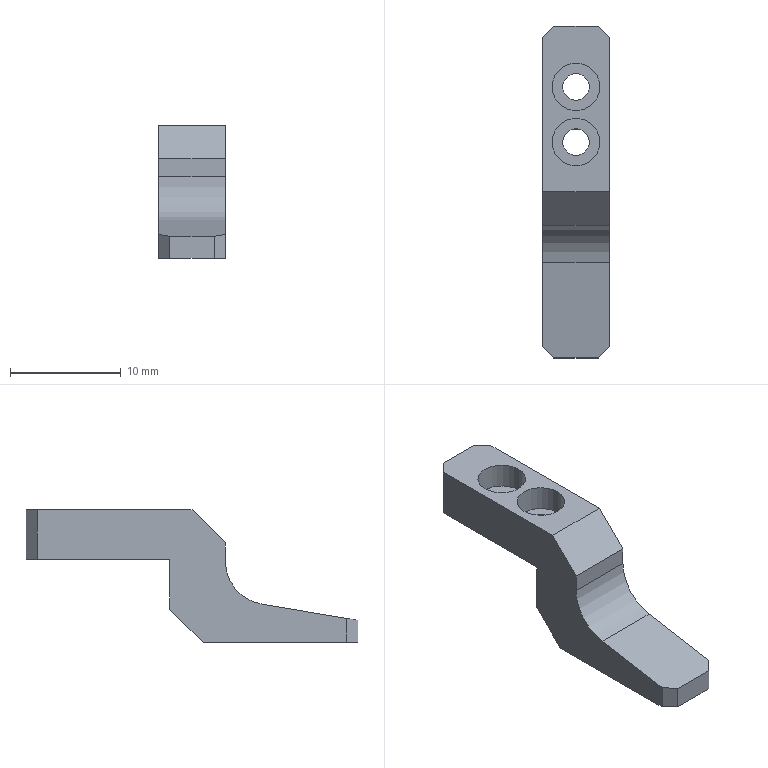Part | STEP file | 0-19-03 Finger | 1 solid | 27 faces | box 6 x 30 x 12 mm | volume 793.591 mm3 | plane 18 | cylinder 9 | commonest cylinder face diameters 2.4 x4 4.3 x4 8 x1